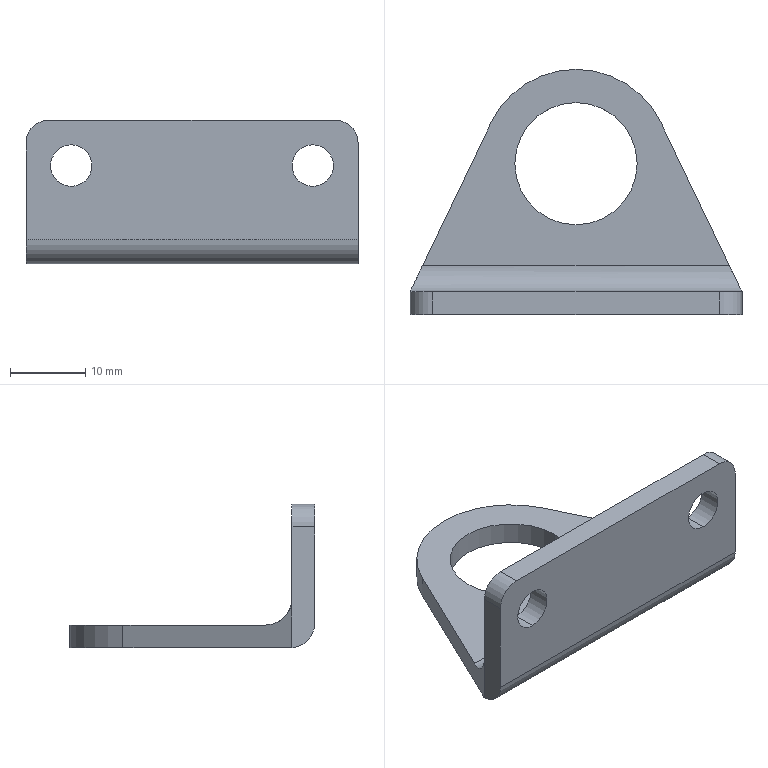Part | STEP file | 1 solid | 20 faces | box 44 x 32.5 x 19 mm | volume 4333 mm3 | cylinder 11 | plane 9 | commonest cylinder face diameters 5.5 x4 6 x2 16.2 x2 6.4 x1 7 x1 25 x1